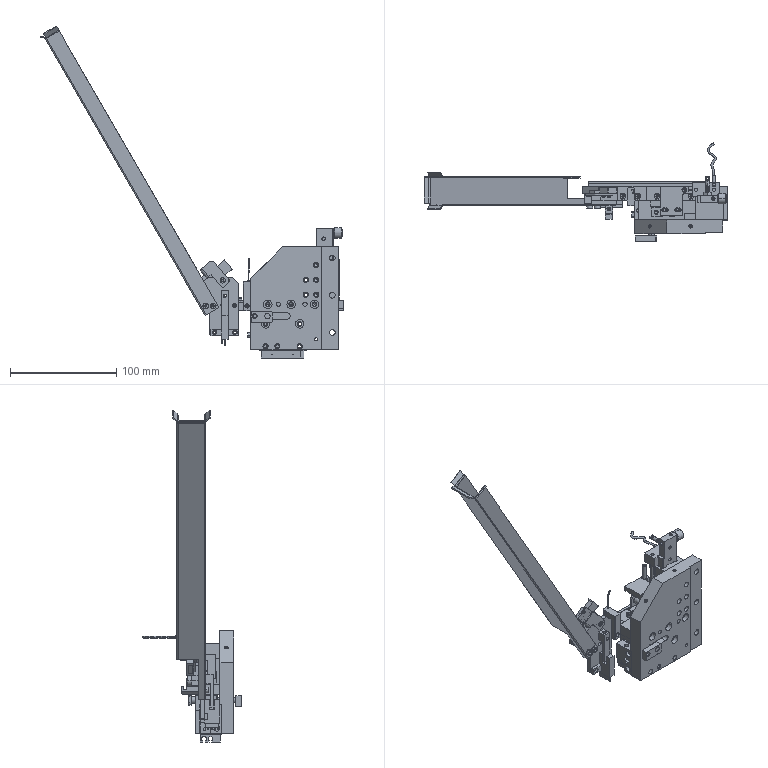Part | NX | 53 solids | 2464 faces | box 285.673 x 92.598 x 312.186 mm | volume 229423 mm3 | plane 1600 | cylinder 595 | cone 238 | spline 18 | torus 12 | sphere 1 | commonest cylinder face diameters 2.5 x102 4 x86 3 x56 3.3 x38 5 x38 3.5 x34